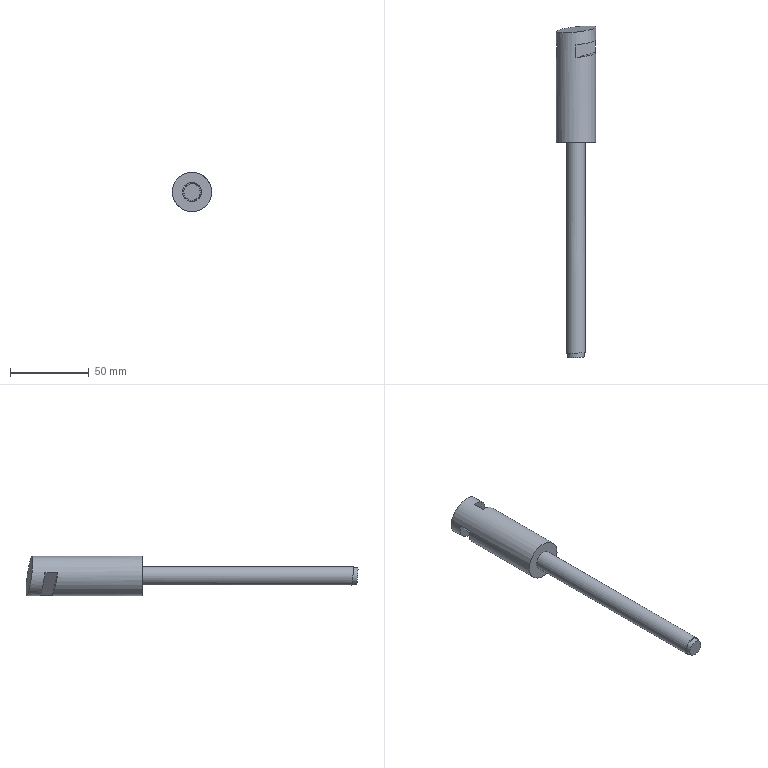Part | STEP file | solid 150 | 1 solid | 13 faces | box 25 x 210.948 x 25 mm | volume 49531 mm3 | plane 8 | spline 3 | cylinder 2 | commonest cylinder face diameters 12 x1 25 x1